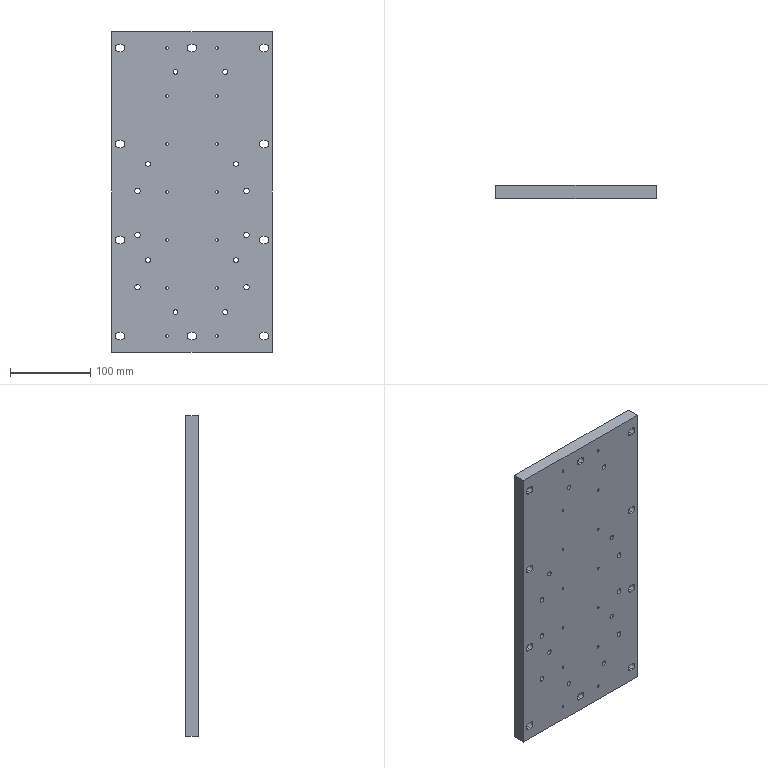Part | NX | 1 solid | 152 faces | box 200 x 16 x 400 mm | volume 1256403 mm3 | cylinder 86 | cone 40 | plane 26 | commonest cylinder face diameters 9 x30 3.3 x28 6 x16 6.8 x12